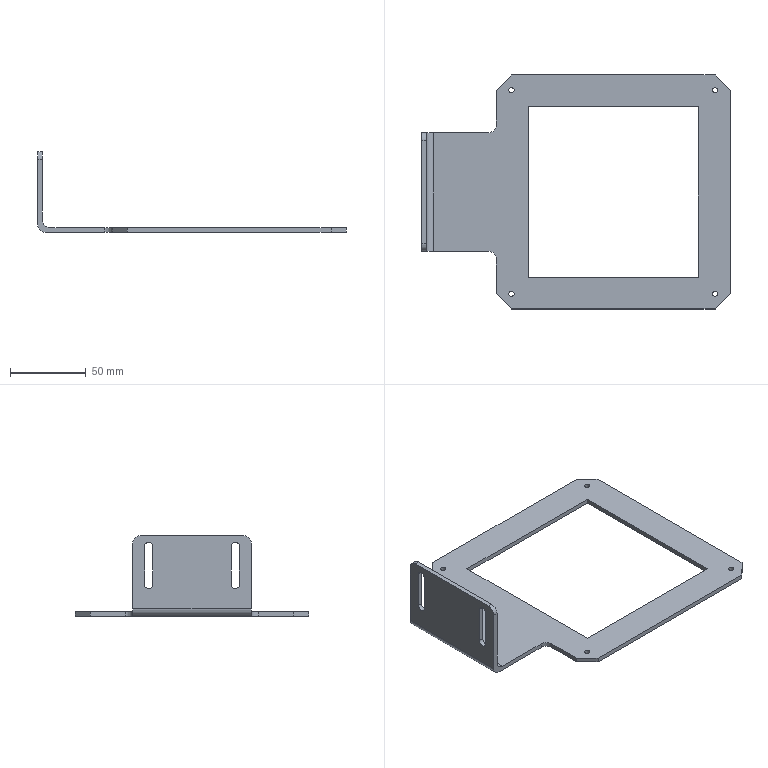Part | STEP file | 11-FG-S02711 | 1 solid | 44 faces | box 203 x 154 x 53 mm | volume 54999 mm3 | plane 24 | cylinder 20 | commonest cylinder face diameters 3.5 x8 5.5 x6 10 x6
STEP:
#1=CARTESIAN_POINT('',(145.75,144.,3.));
#2=VERTEX_POINT('',#1);
#3=CARTESIAN_POINT('',(142.25,144.,3.));
#4=VERTEX_POINT('',#3);
#5=CARTESIAN_POINT('',(144.,144.,3.));
#6=DIRECTION('',(0.,0.,-1.));
#7=DIRECTION('',(-1.,0.,0.));
#8=AXIS2_PLACEMENT_3D('',#5,#6,#7);
#9=CIRCLE('',#8,1.75);
#10=EDGE_CURVE('',#2,#4,#9,.T.);
#11=ORIENTED_EDGE('',*,*,#10,.F.);
#12=CARTESIAN_POINT('',(145.75,144.,0.));
#13=VERTEX_POINT('',#12);
#14=CARTESIAN_POINT('',(145.75,144.,10.));
#15=DIRECTION('',(0.,0.,-1.));
#16=VECTOR('',#15,1000.);
#17=LINE('',#14,#16);
#18=EDGE_CURVE('',#2,#13,#17,.T.);
#19=ORIENTED_EDGE('',*,*,#18,.T.);
#20=CARTESIAN_POINT('',(142.25,144.,0.));
#21=VERTEX_POINT('',#20);
#22=CARTESIAN_POINT('',(144.,144.,0.));
#23=DIRECTION('',(0.,0.,-1.));
#24=DIRECTION('',(-1.,0.,0.));
#25=AXIS2_PLACEMENT_3D('',#22,#23,#24);
#26=CIRCLE('',#25,1.75);
#27=EDGE_CURVE('',#13,#21,#26,.T.);
#28=ORIENTED_EDGE('',*,*,#27,.T.);
#29=CARTESIAN_POINT('',(142.25,144.,10.));
#30=DIRECTION('',(0.,0.,-1.));
#31=VECTOR('',#30,1000.);
#32=LINE('',#29,#31);
#33=EDGE_CURVE('',#4,#21,#32,.T.);
#34=ORIENTED_EDGE('',*,*,#33,.F.);
#35=EDGE_LOOP('',(#11,#19,#28,#34));
#36=FACE_OUTER_BOUND('',#35,.T.);
#37=CARTESIAN_POINT('',(144.,144.,10.));
#38=DIRECTION('',(0.,0.,-1.));
#39=DIRECTION('',(-1.,0.,0.));
#40=AXIS2_PLACEMENT_3D('',#37,#38,#39);
#41=CYLINDRICAL_SURFACE('',#40,1.75);
#42=ADVANCED_FACE('',(#36),#41,.F.);
#43=CARTESIAN_POINT('',(145.75,10.,3.));
#44=VERTEX_POINT('',#43);
#45=CARTESIAN_POINT('',(142.25,10.,3.));
#46=VERTEX_POINT('',#45);
#47=CARTESIAN_POINT('',(144.,10.,3.));
#48=DIRECTION('',(0.,0.,-1.));
#49=DIRECTION('',(-1.,0.,0.));
#50=AXIS2_PLACEMENT_3D('',#47,#48,#49);
#51=CIRCLE('',#50,1.75);
#52=EDGE_CURVE('',#44,#46,#51,.T.);
#53=ORIENTED_EDGE('',*,*,#52,.F.);
#54=CARTESIAN_POINT('',(145.75,10.,0.));
#55=VERTEX_POINT('',#54);
#56=CARTESIAN_POINT('',(145.75,10.,10.));
#57=DIRECTION('',(0.,0.,-1.));
#58=VECTOR('',#57,1000.);
#59=LINE('',#56,#58);
#60=EDGE_CURVE('',#44,#55,#59,.T.);
#61=ORIENTED_EDGE('',*,*,#60,.T.);
#62=CARTESIAN_POINT('',(142.25,10.,0.));
#63=VERTEX_POINT('',#62);
#64=CARTESIAN_POINT('',(144.,10.,0.));
#65=DIRECTION('',(0.,0.,-1.));
#66=DIRECTION('',(-1.,0.,0.));
#67=AXIS2_PLACEMENT_3D('',#64,#65,#66);
#68=CIRCLE('',#67,1.75);
#69=EDGE_CURVE('',#55,#63,#68,.T.);
#70=ORIENTED_EDGE('',*,*,#69,.T.);
#71=CARTESIAN_POINT('',(142.25,10.,10.));
#72=DIRECTION('',(0.,0.,-1.));
#73=VECTOR('',#72,1000.);
#74=LINE('',#71,#73);
#75=EDGE_CURVE('',#46,#63,#74,.T.);
#76=ORIENTED_EDGE('',*,*,#75,.F.);
#77=EDGE_LOOP('',(#53,#61,#70,#76));
#78=FACE_OUTER_BOUND('',#77,.T.);
#79=CARTESIAN_POINT('',(144.,10.,10.));
#80=DIRECTION('',(0.,0.,-1.));
#81=DIRECTION('',(-1.,0.,0.));
#82=AXIS2_PLACEMENT_3D('',#79,#80,#81);
#83=CYLINDRICAL_SURFACE('',#82,1.75);
#84=ADVANCED_FACE('',(#78),#83,.F.);
#85=CARTESIAN_POINT('',(11.75,10.,3.));
#86=VERTEX_POINT('',#85);
#87=CARTESIAN_POINT('',(8.25,10.,3.));
#88=VERTEX_POINT('',#87);
#89=CARTESIAN_POINT('',(10.,10.,3.));
#90=DIRECTION('',(0.,0.,-1.));
#91=DIRECTION('',(-1.,0.,0.));
#92=AXIS2_PLACEMENT_3D('',#89,#90,#91);
#93=CIRCLE('',#92,1.75);
#94=EDGE_CURVE('',#86,#88,#93,.T.);
#95=ORIENTED_EDGE('',*,*,#94,.F.);
#96=CARTESIAN_POINT('',(11.75,10.,0.));
#97=VERTEX_POINT('',#96);
#98=CARTESIAN_POINT('',(11.75,10.,10.));
#99=DIRECTION('',(0.,0.,-1.));
#100=VECTOR('',#99,1000.);
#101=LINE('',#98,#100);
#102=EDGE_CURVE('',#86,#97,#101,.T.);
#103=ORIENTED_EDGE('',*,*,#102,.T.);
#104=CARTESIAN_POINT('',(8.25,10.,0.));
#105=VERTEX_POINT('',#104);
#106=CARTESIAN_POINT('',(10.,10.,0.));
#107=DIRECTION('',(0.,0.,-1.));
#108=DIRECTION('',(-1.,0.,0.));
#109=AXIS2_PLACEMENT_3D('',#106,#107,#108);
#110=CIRCLE('',#109,1.75);
#111=EDGE_CURVE('',#97,#105,#110,.T.);
#112=ORIENTED_EDGE('',*,*,#111,.T.);
#113=CARTESIAN_POINT('',(8.25,10.,10.));
#114=DIRECTION('',(0.,0.,-1.));
#115=VECTOR('',#114,1000.);
#116=LINE('',#113,#115);
#117=EDGE_CURVE('',#88,#105,#116,.T.);
#118=ORIENTED_EDGE('',*,*,#117,.F.);
#119=EDGE_LOOP('',(#95,#103,#112,#118));
#120=FACE_OUTER_BOUND('',#119,.T.);
#121=CARTESIAN_POINT('',(10.,10.,10.));
#122=DIRECTION('',(0.,0.,-1.));
#123=DIRECTION('',(-1.,0.,0.));
#124=AXIS2_PLACEMENT_3D('',#121,#122,#123);
#125=CYLINDRICAL_SURFACE('',#124,1.75);
#126=ADVANCED_FACE('',(#120),#125,.F.);
#127=CARTESIAN_POINT('',(11.75,144.,3.));
#128=VERTEX_POINT('',#127);
#129=CARTESIAN_POINT('',(8.25,144.,3.));
#130=VERTEX_POINT('',#129);
#131=CARTESIAN_POINT('',(10.,144.,3.));
#132=DIRECTION('',(0.,0.,-1.));
#133=DIRECTION('',(-1.,0.,0.));
#134=AXIS2_PLACEMENT_3D('',#131,#132,#133);
#135=CIRCLE('',#134,1.75);
#136=EDGE_CURVE('',#128,#130,#135,.T.);
#137=ORIENTED_EDGE('',*,*,#136,.F.);
#138=CARTESIAN_POINT('',(11.75,144.,0.));
#139=VERTEX_POINT('',#138);
#140=CARTESIAN_POINT('',(11.75,144.,10.));
#141=DIRECTION('',(0.,0.,-1.));
#142=VECTOR('',#141,1000.);
#143=LINE('',#140,#142);
#144=EDGE_CURVE('',#128,#139,#143,.T.);
#145=ORIENTED_EDGE('',*,*,#144,.T.);
#146=CARTESIAN_POINT('',(8.25,144.,0.));
#147=VERTEX_POINT('',#146);
#148=CARTESIAN_POINT('',(10.,144.,0.));
#149=DIRECTION('',(0.,0.,-1.));
#150=DIRECTION('',(-1.,0.,0.));
#151=AXIS2_PLACEMENT_3D('',#148,#149,#150);
#152=CIRCLE('',#151,1.75);
#153=EDGE_CURVE('',#139,#147,#152,.T.);
#154=ORIENTED_EDGE('',*,*,#153,.T.);
#155=CARTESIAN_POINT('',(8.25,144.,10.));
#156=DIRECTION('',(0.,0.,-1.));
#157=VECTOR('',#156,1000.);
#158=LINE('',#155,#157);
#159=EDGE_CURVE('',#130,#147,#158,.T.);
#160=ORIENTED_EDGE('',*,*,#159,.F.);
#161=EDGE_LOOP('',(#137,#145,#154,#160));
#162=FACE_OUTER_BOUND('',#161,.T.);
#163=CARTESIAN_POINT('',(10.,144.,10.));
#164=DIRECTION('',(0.,0.,-1.));
#165=DIRECTION('',(-1.,0.,0.));
#166=AXIS2_PLACEMENT_3D('',#163,#164,#165);
#167=CYLINDRICAL_SURFACE('',#166,1.75);
#168=ADVANCED_FACE('',(#162),#167,.F.);
#169=CARTESIAN_POINT('',(-46.,105.5,48.75));
#170=VERTEX_POINT('',#169);
#171=CARTESIAN_POINT('',(-46.,108.25,46.));
#172=VERTEX_POINT('',#171);
#173=CARTESIAN_POINT('',(-46.,105.5,46.));
#174=DIRECTION('',(-1.,0.,0.));
#175=DIRECTION('',(0.,0.,1.));
#176=AXIS2_PLACEMENT_3D('',#173,#174,#175);
#177=CIRCLE('',#176,2.75);
#178=EDGE_CURVE('',#170,#172,#177,.T.);
#179=ORIENTED_EDGE('',*,*,#178,.F.);
#180=CARTESIAN_POINT('',(-49.,105.5,48.75));
#181=VERTEX_POINT('',#180);
#182=CARTESIAN_POINT('',(1.,105.5,48.75));
#183=DIRECTION('',(-1.,0.,0.));
#184=VECTOR('',#183,1000.);
#185=LINE('',#182,#184);
#186=EDGE_CURVE('',#170,#181,#185,.T.);
#187=ORIENTED_EDGE('',*,*,#186,.T.);
#188=CARTESIAN_POINT('',(-49.,108.25,46.));
#189=VERTEX_POINT('',#188);
#190=CARTESIAN_POINT('',(-49.,105.5,46.));
#191=DIRECTION('',(-1.,0.,0.));
#192=DIRECTION('',(0.,0.,1.));
#193=AXIS2_PLACEMENT_3D('',#190,#191,#192);
#194=CIRCLE('',#193,2.75);
#195=EDGE_CURVE('',#181,#189,#194,.T.);
#196=ORIENTED_EDGE('',*,*,#195,.T.);
#197=CARTESIAN_POINT('',(1.,108.25,46.));
#198=DIRECTION('',(-1.,0.,0.));
#199=VECTOR('',#198,1000.);
#200=LINE('',#197,#199);
#201=EDGE_CURVE('',#172,#189,#200,.T.);
#202=ORIENTED_EDGE('',*,*,#201,.F.);
#203=EDGE_LOOP('',(#179,#187,#196,#202));
#204=FACE_OUTER_BOUND('',#203,.T.);
#205=CARTESIAN_POINT('',(1.,105.5,46.));
#206=DIRECTION('',(-1.,0.,0.));
#207=DIRECTION('',(0.,0.,1.));
#208=AXIS2_PLACEMENT_3D('',#205,#206,#207);
#209=CYLINDRICAL_SURFACE('',#208,2.75);
#210=ADVANCED_FACE('',(#204),#209,.F.);
#211=CARTESIAN_POINT('',(-46.,48.5,48.75));
#212=VERTEX_POINT('',#211);
#213=CARTESIAN_POINT('',(-46.,51.25,46.));
#214=VERTEX_POINT('',#213);
#215=CARTESIAN_POINT('',(-46.,48.5,46.));
#216=DIRECTION('',(-1.,0.,0.));
#217=DIRECTION('',(0.,0.,1.));
#218=AXIS2_PLACEMENT_3D('',#215,#216,#217);
#219=CIRCLE('',#218,2.75);
#220=EDGE_CURVE('',#212,#214,#219,.T.);
#221=ORIENTED_EDGE('',*,*,#220,.F.);
#222=CARTESIAN_POINT('',(-49.,48.5,48.75));
#223=VERTEX_POINT('',#222);
#224=CARTESIAN_POINT('',(1.,48.5,48.75));
#225=DIRECTION('',(-1.,0.,0.));
#226=VECTOR('',#225,1000.);
#227=LINE('',#224,#226);
#228=EDGE_CURVE('',#212,#223,#227,.T.);
#229=ORIENTED_EDGE('',*,*,#228,.T.);
#230=CARTESIAN_POINT('',(-49.,51.25,46.));
#231=VERTEX_POINT('',#230);
#232=CARTESIAN_POINT('',(-49.,48.5,46.));
#233=DIRECTION('',(-1.,0.,0.));
#234=DIRECTION('',(0.,0.,1.));
#235=AXIS2_PLACEMENT_3D('',#232,#233,#234);
#236=CIRCLE('',#235,2.75);
#237=EDGE_CURVE('',#223,#231,#236,.T.);
#238=ORIENTED_EDGE('',*,*,#237,.T.);
#239=CARTESIAN_POINT('',(1.,51.25,46.));
#240=DIRECTION('',(-1.,0.,0.));
#241=VECTOR('',#240,1000.);
#242=LINE('',#239,#241);
#243=EDGE_CURVE('',#214,#231,#242,.T.);
#244=ORIENTED_EDGE('',*,*,#243,.F.);
#245=EDGE_LOOP('',(#221,#229,#238,#244));
#246=FACE_OUTER_BOUND('',#245,.T.);
#247=CARTESIAN_POINT('',(1.,48.5,46.));
#248=DIRECTION('',(-1.,0.,0.));
#249=DIRECTION('',(0.,0.,1.));
#250=AXIS2_PLACEMENT_3D('',#247,#248,#249);
#251=CYLINDRICAL_SURFACE('',#250,2.75);
#252=ADVANCED_FACE('',(#246),#251,.F.);
#253=CARTESIAN_POINT('',(144.,144.,3.));
#254=DIRECTION('',(0.,0.,-1.));
#255=DIRECTION('',(-1.,0.,0.));
#256=AXIS2_PLACEMENT_3D('',#253,#254,#255);
#257=CIRCLE('',#256,1.75);
#258=EDGE_CURVE('',#4,#2,#257,.T.);
#259=ORIENTED_EDGE('',*,*,#258,.T.);
#260=ORIENTED_EDGE('',*,*,#10,.T.);
#261=EDGE_LOOP('',(#259,#260));
#262=FACE_BOUND('',#261,.T.);
#263=CARTESIAN_POINT('',(144.,10.,3.));
#264=DIRECTION('',(0.,0.,-1.));
#265=DIRECTION('',(-1.,0.,0.));
#266=AXIS2_PLACEMENT_3D('',#263,#264,#265);
#267=CIRCLE('',#266,1.75);
#268=EDGE_CURVE('',#46,#44,#267,.T.);
#269=ORIENTED_EDGE('',*,*,#268,.T.);
#270=ORIENTED_EDGE('',*,*,#52,.T.);
#271=EDGE_LOOP('',(#269,#270));
#272=FACE_BOUND('',#271,.T.);
#273=CARTESIAN_POINT('',(10.,10.,3.));
#274=DIRECTION('',(0.,0.,-1.));
#275=DIRECTION('',(-1.,0.,0.));
#276=AXIS2_PLACEMENT_3D('',#273,#274,#275);
#277=CIRCLE('',#276,1.75);
#278=EDGE_CURVE('',#88,#86,#277,.T.);
#279=ORIENTED_EDGE('',*,*,#278,.T.);
#280=ORIENTED_EDGE('',*,*,#94,.T.);
#281=EDGE_LOOP('',(#279,#280));
#282=FACE_BOUND('',#281,.T.);
#283=CARTESIAN_POINT('',(10.,144.,3.));
#284=DIRECTION('',(0.,0.,-1.));
#285=DIRECTION('',(-1.,0.,0.));
#286=AXIS2_PLACEMENT_3D('',#283,#284,#285);
#287=CIRCLE('',#286,1.75);
#288=EDGE_CURVE('',#130,#128,#287,.T.);
#289=ORIENTED_EDGE('',*,*,#288,.T.);
#290=ORIENTED_EDGE('',*,*,#136,.T.);
#291=EDGE_LOOP('',(#289,#290));
#292=FACE_BOUND('',#291,.T.);
#293=CARTESIAN_POINT('',(21.,133.,3.));
#294=VERTEX_POINT('',#293);
#295=CARTESIAN_POINT('',(21.,21.,3.));
#296=VERTEX_POINT('',#295);
#297=CARTESIAN_POINT('',(21.,21.,3.));
#298=DIRECTION('',(0.,-1.,0.));
#299=VECTOR('',#298,1000.);
#300=LINE('',#297,#299);
#301=EDGE_CURVE('',#294,#296,#300,.T.);
#302=ORIENTED_EDGE('',*,*,#301,.F.);
#303=CARTESIAN_POINT('',(133.,133.,3.));
#304=VERTEX_POINT('',#303);
#305=CARTESIAN_POINT('',(21.,133.,3.));
#306=DIRECTION('',(-1.,0.,0.));
#307=VECTOR('',#306,1000.);
#308=LINE('',#305,#307);
#309=EDGE_CURVE('',#304,#294,#308,.T.);
#310=ORIENTED_EDGE('',*,*,#309,.F.);
#311=CARTESIAN_POINT('',(133.,21.,3.));
#312=VERTEX_POINT('',#311);
#313=CARTESIAN_POINT('',(133.,21.,3.));
#314=DIRECTION('',(0.,1.,0.));
#315=VECTOR('',#314,1000.);
#316=LINE('',#313,#315);
#317=EDGE_CURVE('',#312,#304,#316,.T.);
#318=ORIENTED_EDGE('',*,*,#317,.F.);
#319=CARTESIAN_POINT('',(21.,21.,3.));
#320=DIRECTION('',(1.,0.,0.));
#321=VECTOR('',#320,1000.);
#322=LINE('',#319,#321);
#323=EDGE_CURVE('',#296,#312,#322,.T.);
#324=ORIENTED_EDGE('',*,*,#323,.F.);
#325=EDGE_LOOP('',(#302,#310,#318,#324));
#326=FACE_BOUND('',#325,.T.);
#327=CARTESIAN_POINT('',(-41.,116.,3.));
#328=VERTEX_POINT('',#327);
#329=CARTESIAN_POINT('',(-5.,116.,3.));
#330=VERTEX_POINT('',#329);
#331=CARTESIAN_POINT('',(-49.,116.,3.));
#332=DIRECTION('',(1.,0.,0.));
#333=VECTOR('',#332,1000.);
#334=LINE('',#331,#333);
#335=EDGE_CURVE('',#328,#330,#334,.T.);
#336=ORIENTED_EDGE('',*,*,#335,.F.);
#337=CARTESIAN_POINT('',(-41.,38.,3.));
#338=VERTEX_POINT('',#337);
#339=CARTESIAN_POINT('',(-41.,38.,3.));
#340=DIRECTION('',(0.,-1.,0.));
#341=VECTOR('',#340,1000.);
#342=LINE('',#339,#341);
#343=EDGE_CURVE('',#328,#338,#342,.T.);
#344=ORIENTED_EDGE('',*,*,#343,.T.);
#345=CARTESIAN_POINT('',(-5.,38.,3.));
#346=VERTEX_POINT('',#345);
#347=CARTESIAN_POINT('',(-49.,38.,3.));
#348=DIRECTION('',(1.,0.,0.));
#349=VECTOR('',#348,1000.);
#350=LINE('',#347,#349);
#351=EDGE_CURVE('',#338,#346,#350,.T.);
#352=ORIENTED_EDGE('',*,*,#351,.T.);
#353=CARTESIAN_POINT('',(0.,33.,3.));
#354=VERTEX_POINT('',#353);
#355=CARTESIAN_POINT('',(-5.,33.,3.));
#356=DIRECTION('',(0.,0.,-1.));
#357=DIRECTION('',(-1.,0.,0.));
#358=AXIS2_PLACEMENT_3D('',#355,#356,#357);
#359=CIRCLE('',#358,5.);
#360=EDGE_CURVE('',#346,#354,#359,.T.);
#361=ORIENTED_EDGE('',*,*,#360,.T.);
#362=CARTESIAN_POINT('',(0.,10.,3.));
#363=VERTEX_POINT('',#362);
#364=CARTESIAN_POINT('',(0.,0.,3.));
#365=DIRECTION('',(0.,-1.,0.));
#366=VECTOR('',#365,1000.);
#367=LINE('',#364,#366);
#368=EDGE_CURVE('',#354,#363,#367,.T.);
#369=ORIENTED_EDGE('',*,*,#368,.T.);
#370=CARTESIAN_POINT('',(10.,0.,3.));
#371=VERTEX_POINT('',#370);
#372=CARTESIAN_POINT('',(10.,0.,3.));
#373=DIRECTION('',(0.7071,-0.7071,0.));
#374=VECTOR('',#373,1000.);
#375=LINE('',#372,#374);
#376=EDGE_CURVE('',#363,#371,#375,.T.);
#377=ORIENTED_EDGE('',*,*,#376,.T.);
#378=CARTESIAN_POINT('',(144.,0.,3.));
#379=VERTEX_POINT('',#378);
#380=CARTESIAN_POINT('',(0.,0.,3.));
#381=DIRECTION('',(1.,0.,0.));
#382=VECTOR('',#381,1000.);
#383=LINE('',#380,#382);
#384=EDGE_CURVE('',#371,#379,#383,.T.);
#385=ORIENTED_EDGE('',*,*,#384,.T.);
#386=CARTESIAN_POINT('',(154.,10.,3.));
#387=VERTEX_POINT('',#386);
#388=CARTESIAN_POINT('',(154.,10.,3.));
#389=DIRECTION('',(0.7071,0.7071,0.));
#390=VECTOR('',#389,1000.);
#391=LINE('',#388,#390);
#392=EDGE_CURVE('',#379,#387,#391,.T.);
#393=ORIENTED_EDGE('',*,*,#392,.T.);
#394=CARTESIAN_POINT('',(154.,144.,3.));
#395=VERTEX_POINT('',#394);
#396=CARTESIAN_POINT('',(154.,0.,3.));
#397=DIRECTION('',(0.,1.,0.));
#398=VECTOR('',#397,1000.);
#399=LINE('',#396,#398);
#400=EDGE_CURVE('',#387,#395,#399,.T.);
#401=ORIENTED_EDGE('',*,*,#400,.T.);
#402=CARTESIAN_POINT('',(144.,154.,3.));
#403=VERTEX_POINT('',#402);
#404=CARTESIAN_POINT('',(144.,154.,3.));
#405=DIRECTION('',(-0.7071,0.7071,0.));
#406=VECTOR('',#405,1000.);
#407=LINE('',#404,#406);
#408=EDGE_CURVE('',#395,#403,#407,.T.);
#409=ORIENTED_EDGE('',*,*,#408,.T.);
#410=CARTESIAN_POINT('',(10.,154.,3.));
#411=VERTEX_POINT('',#410);
#412=CARTESIAN_POINT('',(0.,154.,3.));
#413=DIRECTION('',(-1.,0.,0.));
#414=VECTOR('',#413,1000.);
#415=LINE('',#412,#414);
#416=EDGE_CURVE('',#403,#411,#415,.T.);
#417=ORIENTED_EDGE('',*,*,#416,.T.);
#418=CARTESIAN_POINT('',(0.,144.,3.));
#419=VERTEX_POINT('',#418);
#420=CARTESIAN_POINT('',(0.,144.,3.));
#421=DIRECTION('',(-0.7071,-0.7071,0.));
#422=VECTOR('',#421,1000.);
#423=LINE('',#420,#422);
#424=EDGE_CURVE('',#411,#419,#423,.T.);
#425=ORIENTED_EDGE('',*,*,#424,.T.);
#426=CARTESIAN_POINT('',(0.,121.,3.));
#427=VERTEX_POINT('',#426);
#428=CARTESIAN_POINT('',(0.,0.,3.));
#429=DIRECTION('',(0.,-1.,0.));
#430=VECTOR('',#429,1000.);
#431=LINE('',#428,#430);
#432=EDGE_CURVE('',#419,#427,#431,.T.);
#433=ORIENTED_EDGE('',*,*,#432,.T.);
#434=CARTESIAN_POINT('',(-5.,121.,3.));
#435=DIRECTION('',(0.,0.,-1.));
#436=DIRECTION('',(-1.,0.,0.));
#437=AXIS2_PLACEMENT_3D('',#434,#435,#436);
#438=CIRCLE('',#437,5.);
#439=EDGE_CURVE('',#427,#330,#438,.T.);
#440=ORIENTED_EDGE('',*,*,#439,.T.);
#441=EDGE_LOOP('',(#336,#344,#352,#361,#369,#377,#385,#393,#401,#409,#417,#425,#433,#440));
#442=FACE_OUTER_BOUND('',#441,.T.);
#443=CARTESIAN_POINT('',(0.,0.,3.));
#444=DIRECTION('',(0.,0.,-1.));
#445=DIRECTION('',(-1.,0.,0.));
#446=AXIS2_PLACEMENT_3D('',#443,#444,#445);
#447=PLANE('',#446);
#448=ADVANCED_FACE('',(#262,#272,#282,#292,#326,#442),#447,.F.);
#449=CARTESIAN_POINT('',(0.,144.,0.));
#450=VERTEX_POINT('',#449);
#451=CARTESIAN_POINT('',(0.,121.,0.));
#452=VERTEX_POINT('',#451);
#453=CARTESIAN_POINT('',(0.,0.,0.));
#454=DIRECTION('',(0.,-1.,0.));
#455=VECTOR('',#454,1000.);
#456=LINE('',#453,#455);
#457=EDGE_CURVE('',#450,#452,#456,.T.);
#458=ORIENTED_EDGE('',*,*,#457,.T.);
#459=CARTESIAN_POINT('',(0.,121.,3.));
#460=DIRECTION('',(0.,0.,1.));
#461=VECTOR('',#460,1000.);
#462=LINE('',#459,#461);
#463=EDGE_CURVE('',#452,#427,#462,.T.);
#464=ORIENTED_EDGE('',*,*,#463,.T.);
#465=ORIENTED_EDGE('',*,*,#432,.F.);
#466=CARTESIAN_POINT('',(0.,144.,3.));
#467=DIRECTION('',(0.,0.,-1.));
#468=VECTOR('',#467,1000.);
#469=LINE('',#466,#468);
#470=EDGE_CURVE('',#419,#450,#469,.T.);
#471=ORIENTED_EDGE('',*,*,#470,.T.);
#472=EDGE_LOOP('',(#458,#464,#465,#471));
#473=FACE_OUTER_BOUND('',#472,.T.);
#474=CARTESIAN_POINT('',(0.,0.,3.));
#475=DIRECTION('',(1.,0.,0.));
#476=DIRECTION('',(0.,0.,-1.));
#477=AXIS2_PLACEMENT_3D('',#474,#475,#476);
#478=PLANE('',#477);
#479=ADVANCED_FACE('',(#473),#478,.F.);
#480=ORIENTED_EDGE('',*,*,#368,.F.);
#481=CARTESIAN_POINT('',(0.,33.,0.));
#482=VERTEX_POINT('',#481);
#483=CARTESIAN_POINT('',(0.,33.,0.));
#484=DIRECTION('',(0.,0.,-1.));
#485=VECTOR('',#484,1000.);
#486=LINE('',#483,#485);
#487=EDGE_CURVE('',#354,#482,#486,.T.);
#488=ORIENTED_EDGE('',*,*,#487,.T.);
#489=CARTESIAN_POINT('',(0.,10.,0.));
#490=VERTEX_POINT('',#489);
#491=CARTESIAN_POINT('',(0.,0.,0.));
#492=DIRECTION('',(0.,-1.,0.));
#493=VECTOR('',#492,1000.);
#494=LINE('',#491,#493);
#495=EDGE_CURVE('',#482,#490,#494,.T.);
#496=ORIENTED_EDGE('',*,*,#495,.T.);
#497=CARTESIAN_POINT('',(0.,10.,3.));
#498=DIRECTION('',(0.,0.,1.));
#499=VECTOR('',#498,1000.);
#500=LINE('',#497,#499);
#501=EDGE_CURVE('',#490,#363,#500,.T.);
#502=ORIENTED_EDGE('',*,*,#501,.T.);
#503=EDGE_LOOP('',(#480,#488,#496,#502));
#504=FACE_OUTER_BOUND('',#503,.T.);
#505=CARTESIAN_POINT('',(0.,0.,3.));
#506=DIRECTION('',(1.,0.,0.));
#507=DIRECTION('',(0.,0.,-1.));
#508=AXIS2_PLACEMENT_3D('',#505,#506,#507);
#509=PLANE('',#508);
#510=ADVANCED_FACE('',(#504),#509,.F.);
#511=CARTESIAN_POINT('',(144.,144.,0.));
#512=DIRECTION('',(0.,0.,-1.));
#513=DIRECTION('',(-1.,0.,0.));
#514=AXIS2_PLACEMENT_3D('',#511,#512,#513);
#515=CIRCLE('',#514,1.75);
#516=EDGE_CURVE('',#21,#13,#515,.T.);
#517=ORIENTED_EDGE('',*,*,#516,.F.);
#518=ORIENTED_EDGE('',*,*,#27,.F.);
#519=EDGE_LOOP('',(#517,#518));
#520=FACE_BOUND('',#519,.T.);
#521=CARTESIAN_POINT('',(144.,10.,0.));
#522=DIRECTION('',(0.,0.,-1.));
#523=DIRECTION('',(-1.,0.,0.));
#524=AXIS2_PLACEMENT_3D('',#521,#522,#523);
#525=CIRCLE('',#524,1.75);
#526=EDGE_CURVE('',#63,#55,#525,.T.);
#527=ORIENTED_EDGE('',*,*,#526,.F.);
#528=ORIENTED_EDGE('',*,*,#69,.F.);
#529=EDGE_LOOP('',(#527,#528));
#530=FACE_BOUND('',#529,.T.);
#531=CARTESIAN_POINT('',(10.,10.,0.));
#532=DIRECTION('',(0.,0.,-1.));
#533=DIRECTION('',(-1.,0.,0.));
#534=AXIS2_PLACEMENT_3D('',#531,#532,#533);
#535=CIRCLE('',#534,1.75);
#536=EDGE_CURVE('',#105,#97,#535,.T.);
#537=ORIENTED_EDGE('',*,*,#536,.F.);
#538=ORIENTED_EDGE('',*,*,#111,.F.);
#539=EDGE_LOOP('',(#537,#538));
#540=FACE_BOUND('',#539,.T.);
#541=CARTESIAN_POINT('',(10.,144.,0.));
#542=DIRECTION('',(0.,0.,-1.));
#543=DIRECTION('',(-1.,0.,0.));
#544=AXIS2_PLACEMENT_3D('',#541,#542,#543);
#545=CIRCLE('',#544,1.75);
#546=EDGE_CURVE('',#147,#139,#545,.T.);
#547=ORIENTED_EDGE('',*,*,#546,.F.);
#548=ORIENTED_EDGE('',*,*,#153,.F.);
#549=EDGE_LOOP('',(#547,#548));
#550=FACE_BOUND('',#549,.T.);
#551=CARTESIAN_POINT('',(-44.,38.,0.));
#552=VERTEX_POINT('',#551);
#553=CARTESIAN_POINT('',(-5.,38.,0.));
#554=VERTEX_POINT('',#553);
#555=CARTESIAN_POINT('',(-49.,38.,0.));
#556=DIRECTION('',(1.,0.,0.));
#557=VECTOR('',#556,1000.);
#558=LINE('',#555,#557);
#559=EDGE_CURVE('',#552,#554,#558,.T.);
#560=ORIENTED_EDGE('',*,*,#559,.F.);
#561=CARTESIAN_POINT('',(-44.,116.,0.));
#562=VERTEX_POINT('',#561);
#563=CARTESIAN_POINT('',(-44.,0.,0.));
#564=DIRECTION('',(0.,1.,0.));
#565=VECTOR('',#564,1000.);
#566=LINE('',#563,#565);
#567=EDGE_CURVE('',#552,#562,#566,.T.);
#568=ORIENTED_EDGE('',*,*,#567,.T.);
#569=CARTESIAN_POINT('',(-5.,116.,0.));
#570=VERTEX_POINT('',#569);
#571=CARTESIAN_POINT('',(-49.,116.,0.));
#572=DIRECTION('',(1.,0.,0.));
#573=VECTOR('',#572,1000.);
#574=LINE('',#571,#573);
#575=EDGE_CURVE('',#562,#570,#574,.T.);
#576=ORIENTED_EDGE('',*,*,#575,.T.);
#577=CARTESIAN_POINT('',(-5.,121.,0.));
#578=DIRECTION('',(0.,0.,1.));
#579=DIRECTION('',(-1.,0.,0.));
#580=AXIS2_PLACEMENT_3D('',#577,#578,#579);
#581=CIRCLE('',#580,5.);
#582=EDGE_CURVE('',#570,#452,#581,.T.);
#583=ORIENTED_EDGE('',*,*,#582,.T.);
#584=ORIENTED_EDGE('',*,*,#457,.F.);
#585=CARTESIAN_POINT('',(10.,154.,0.));
#586=VERTEX_POINT('',#585);
#587=CARTESIAN_POINT('',(-72.,72.,0.));
#588=DIRECTION('',(0.7071,0.7071,0.));
#589=VECTOR('',#588,1000.);
#590=LINE('',#587,#589);
#591=EDGE_CURVE('',#450,#586,#590,.T.);
#592=ORIENTED_EDGE('',*,*,#591,.T.);
#593=CARTESIAN_POINT('',(144.,154.,0.));
#594=VERTEX_POINT('',#593);
#595=CARTESIAN_POINT('',(0.,154.,0.));
#596=DIRECTION('',(-1.,0.,0.));
#597=VECTOR('',#596,1000.);
#598=LINE('',#595,#597);
#599=EDGE_CURVE('',#594,#586,#598,.T.);
#600=ORIENTED_EDGE('',*,*,#599,.F.);
#601=CARTESIAN_POINT('',(154.,144.,0.));
#602=VERTEX_POINT('',#601);
#603=CARTESIAN_POINT('',(149.,149.,0.));
#604=DIRECTION('',(0.7071,-0.7071,0.));
#605=VECTOR('',#604,1000.);
#606=LINE('',#603,#605);
#607=EDGE_CURVE('',#594,#602,#606,.T.);
#608=ORIENTED_EDGE('',*,*,#607,.T.);
#609=CARTESIAN_POINT('',(154.,10.,0.));
#610=VERTEX_POINT('',#609);
#611=CARTESIAN_POINT('',(154.,0.,0.));
#612=DIRECTION('',(0.,1.,0.));
#613=VECTOR('',#612,1000.);
#614=LINE('',#611,#613);
#615=EDGE_CURVE('',#610,#602,#614,.T.);
#616=ORIENTED_EDGE('',*,*,#615,.F.);
#617=CARTESIAN_POINT('',(144.,0.,0.));
#618=VERTEX_POINT('',#617);
#619=CARTESIAN_POINT('',(72.,-72.,0.));
#620=DIRECTION('',(-0.7071,-0.7071,0.));
#621=VECTOR('',#620,1000.);
#622=LINE('',#619,#621);
#623=EDGE_CURVE('',#610,#618,#622,.T.);
#624=ORIENTED_EDGE('',*,*,#623,.T.);
#625=CARTESIAN_POINT('',(10.,0.,0.));
#626=VERTEX_POINT('',#625);
#627=CARTESIAN_POINT('',(0.,0.,0.));
#628=DIRECTION('',(1.,0.,0.));
#629=VECTOR('',#628,1000.);
#630=LINE('',#627,#629);
#631=EDGE_CURVE('',#626,#618,#630,.T.);
#632=ORIENTED_EDGE('',*,*,#631,.F.);
#633=CARTESIAN_POINT('',(5.,5.,0.));
#634=DIRECTION('',(-0.7071,0.7071,0.));
#635=VECTOR('',#634,1000.);
#636=LINE('',#633,#635);
#637=EDGE_CURVE('',#626,#490,#636,.T.);
#638=ORIENTED_EDGE('',*,*,#637,.T.);
#639=ORIENTED_EDGE('',*,*,#495,.F.);
#640=CARTESIAN_POINT('',(-5.,33.,0.));
#641=DIRECTION('',(0.,0.,1.));
#642=DIRECTION('',(-1.,0.,0.));
#643=AXIS2_PLACEMENT_3D('',#640,#641,#642);
#644=CIRCLE('',#643,5.);
#645=EDGE_CURVE('',#482,#554,#644,.T.);
#646=ORIENTED_EDGE('',*,*,#645,.T.);
#647=EDGE_LOOP('',(#560,#568,#576,#583,#584,#592,#600,#608,#616,#624,#632,#638,#639,#646));
#648=FACE_OUTER_BOUND('',#647,.T.);
#649=CARTESIAN_POINT('',(133.,133.,0.));
#650=VERTEX_POINT('',#649);
#651=CARTESIAN_POINT('',(21.,133.,0.));
#652=VERTEX_POINT('',#651);
#653=CARTESIAN_POINT('',(21.,133.,0.));
#654=DIRECTION('',(-1.,0.,0.));
#655=VECTOR('',#654,1000.);
#656=LINE('',#653,#655);
#657=EDGE_CURVE('',#650,#652,#656,.T.);
#658=ORIENTED_EDGE('',*,*,#657,.T.);
#659=CARTESIAN_POINT('',(21.,21.,0.));
#660=VERTEX_POINT('',#659);
#661=CARTESIAN_POINT('',(21.,21.,0.));
#662=DIRECTION('',(0.,-1.,0.));
#663=VECTOR('',#662,1000.);
#664=LINE('',#661,#663);
#665=EDGE_CURVE('',#652,#660,#664,.T.);
#666=ORIENTED_EDGE('',*,*,#665,.T.);
#667=CARTESIAN_POINT('',(133.,21.,0.));
#668=VERTEX_POINT('',#667);
#669=CARTESIAN_POINT('',(21.,21.,0.));
#670=DIRECTION('',(1.,0.,0.));
#671=VECTOR('',#670,1000.);
#672=LINE('',#669,#671);
#673=EDGE_CURVE('',#660,#668,#672,.T.);
#674=ORIENTED_EDGE('',*,*,#673,.T.);
#675=CARTESIAN_POINT('',(133.,21.,0.));
#676=DIRECTION('',(0.,1.,0.));
#677=VECTOR('',#676,1000.);
#678=LINE('',#675,#677);
#679=EDGE_CURVE('',#668,#650,#678,.T.);
#680=ORIENTED_EDGE('',*,*,#679,.T.);
#681=EDGE_LOOP('',(#658,#666,#674,#680));
#682=FACE_BOUND('',#681,.T.);
#683=CARTESIAN_POINT('',(0.,0.,0.));
#684=DIRECTION('',(0.,0.,-1.));
#685=DIRECTION('',(-1.,0.,0.));
#686=AXIS2_PLACEMENT_3D('',#683,#684,#685);
#687=PLANE('',#686);
#688=ADVANCED_FACE('',(#520,#530,#540,#550,#648,#682),#687,.T.);
#689=ORIENTED_EDGE('',*,*,#384,.F.);
#690=CARTESIAN_POINT('',(10.,0.,3.));
#691=DIRECTION('',(0.,0.,-1.));
#692=VECTOR('',#691,1000.);
#693=LINE('',#690,#692);
#694=EDGE_CURVE('',#371,#626,#693,.T.);
#695=ORIENTED_EDGE('',*,*,#694,.T.);
#696=ORIENTED_EDGE('',*,*,#631,.T.);
#697=CARTESIAN_POINT('',(144.,0.,3.));
#698=DIRECTION('',(0.,0.,1.));
#699=VECTOR('',#698,1000.);
#700=LINE('',#697,#699);
#701=EDGE_CURVE('',#618,#379,#700,.T.);
#702=ORIENTED_EDGE('',*,*,#701,.T.);
#703=EDGE_LOOP('',(#689,#695,#696,#702));
#704=FACE_OUTER_BOUND('',#703,.T.);
#705=CARTESIAN_POINT('',(0.,0.,3.));
#706=DIRECTION('',(0.,1.,0.));
#707=DIRECTION('',(0.,0.,1.));
#708=AXIS2_PLACEMENT_3D('',#705,#706,#707);
#709=PLANE('',#708);
#710=ADVANCED_FACE('',(#704),#709,.F.);
#711=ORIENTED_EDGE('',*,*,#615,.T.);
#712=CARTESIAN_POINT('',(154.,144.,3.));
#713=DIRECTION('',(0.,0.,1.));
#714=VECTOR('',#713,1000.);
#715=LINE('',#712,#714);
#716=EDGE_CURVE('',#602,#395,#715,.T.);
#717=ORIENTED_EDGE('',*,*,#716,.T.);
#718=ORIENTED_EDGE('',*,*,#400,.F.);
#719=CARTESIAN_POINT('',(154.,10.,3.));
#720=DIRECTION('',(0.,0.,-1.));
#721=VECTOR('',#720,1000.);
#722=LINE('',#719,#721);
#723=EDGE_CURVE('',#387,#610,#722,.T.);
#724=ORIENTED_EDGE('',*,*,#723,.T.);
#725=EDGE_LOOP('',(#711,#717,#718,#724));
#726=FACE_OUTER_BOUND('',#725,.T.);
#727=CARTESIAN_POINT('',(154.,0.,3.));
#728=DIRECTION('',(-1.,0.,0.));
#729=DIRECTION('',(0.,0.,1.));
#730=AXIS2_PLACEMENT_3D('',#727,#728,#729);
#731=PLANE('',#730);
#732=ADVANCED_FACE('',(#726),#731,.F.);
#733=ORIENTED_EDGE('',*,*,#599,.T.);
#734=CARTESIAN_POINT('',(10.,154.,3.));
#735=DIRECTION('',(0.,0.,1.));
#736=VECTOR('',#735,1000.);
#737=LINE('',#734,#736);
#738=EDGE_CURVE('',#586,#411,#737,.T.);
#739=ORIENTED_EDGE('',*,*,#738,.T.);
#740=ORIENTED_EDGE('',*,*,#416,.F.);
#741=CARTESIAN_POINT('',(144.,154.,3.));
#742=DIRECTION('',(0.,0.,-1.));
#743=VECTOR('',#742,1000.);
#744=LINE('',#741,#743);
#745=EDGE_CURVE('',#403,#594,#744,.T.);
#746=ORIENTED_EDGE('',*,*,#745,.T.);
#747=EDGE_LOOP('',(#733,#739,#740,#746));
#748=FACE_OUTER_BOUND('',#747,.T.);
#749=CARTESIAN_POINT('',(0.,154.,3.));
#750=DIRECTION('',(0.,-1.,0.));
#751=DIRECTION('',(0.,0.,-1.));
#752=AXIS2_PLACEMENT_3D('',#749,#750,#751);
#753=PLANE('',#752);
#754=ADVANCED_FACE('',(#748),#753,.F.);
#755=ORIENTED_EDGE('',*,*,#665,.F.);
#756=CARTESIAN_POINT('',(21.,133.,3.));
#757=DIRECTION('',(0.,0.,-1.));
#758=VECTOR('',#757,1000.);
#759=LINE('',#756,#758);
#760=EDGE_CURVE('',#294,#652,#759,.T.);
#761=ORIENTED_EDGE('',*,*,#760,.F.);
#762=ORIENTED_EDGE('',*,*,#301,.T.);
#763=CARTESIAN_POINT('',(21.,21.,3.));
#764=DIRECTION('',(0.,0.,-1.));
#765=VECTOR('',#764,1000.);
#766=LINE('',#763,#765);
#767=EDGE_CURVE('',#296,#660,#766,.T.);
#768=ORIENTED_EDGE('',*,*,#767,.T.);
#769=EDGE_LOOP('',(#755,#761,#762,#768));
#770=FACE_OUTER_BOUND('',#769,.T.);
#771=CARTESIAN_POINT('',(21.,21.,3.));
#772=DIRECTION('',(1.,0.,0.));
#773=DIRECTION('',(0.,0.,-1.));
#774=AXIS2_PLACEMENT_3D('',#771,#772,#773);
#775=PLANE('',#774);
#776=ADVANCED_FACE('',(#770),#775,.T.);
#777=ORIENTED_EDGE('',*,*,#673,.F.);
#778=ORIENTED_EDGE('',*,*,#767,.F.);
#779=ORIENTED_EDGE('',*,*,#323,.T.);
#780=CARTESIAN_POINT('',(133.,21.,3.));
#781=DIRECTION('',(0.,0.,-1.));
#782=VECTOR('',#781,1000.);
#783=LINE('',#780,#782);
#784=EDGE_CURVE('',#312,#668,#783,.T.);
#785=ORIENTED_EDGE('',*,*,#784,.T.);
#786=EDGE_LOOP('',(#777,#778,#779,#785));
#787=FACE_OUTER_BOUND('',#786,.T.);
#788=CARTESIAN_POINT('',(21.,21.,3.));
#789=DIRECTION('',(0.,1.,0.));
#790=DIRECTION('',(0.,0.,1.));
#791=AXIS2_PLACEMENT_3D('',#788,#789,#790);
#792=PLANE('',#791);
#793=ADVANCED_FACE('',(#787),#792,.T.);
#794=ORIENTED_EDGE('',*,*,#679,.F.);
#795=ORIENTED_EDGE('',*,*,#784,.F.);
#796=ORIENTED_EDGE('',*,*,#317,.T.);
#797=CARTESIAN_POINT('',(133.,133.,3.));
#798=DIRECTION('',(0.,0.,-1.));
#799=VECTOR('',#798,1000.);
#800=LINE('',#797,#799);
#801=EDGE_CURVE('',#304,#650,#800,.T.);
#802=ORIENTED_EDGE('',*,*,#801,.T.);
#803=EDGE_LOOP('',(#794,#795,#796,#802));
#804=FACE_OUTER_BOUND('',#803,.T.);
#805=CARTESIAN_POINT('',(133.,21.,3.));
#806=DIRECTION('',(-1.,0.,0.));
#807=DIRECTION('',(0.,0.,1.));
#808=AXIS2_PLACEMENT_3D('',#805,#806,#807);
#809=PLANE('',#808);
#810=ADVANCED_FACE('',(#804),#809,.T.);
#811=ORIENTED_EDGE('',*,*,#657,.F.);
#812=ORIENTED_EDGE('',*,*,#801,.F.);
#813=ORIENTED_EDGE('',*,*,#309,.T.);
#814=ORIENTED_EDGE('',*,*,#760,.T.);
#815=EDGE_LOOP('',(#811,#812,#813,#814));
#816=FACE_OUTER_BOUND('',#815,.T.);
#817=CARTESIAN_POINT('',(21.,133.,3.));
#818=DIRECTION('',(0.,-1.,0.));
#819=DIRECTION('',(0.,0.,-1.));
#820=AXIS2_PLACEMENT_3D('',#817,#818,#819);
#821=PLANE('',#820);
#822=ADVANCED_FACE('',(#816),#821,.T.);
#823=CARTESIAN_POINT('',(-46.,38.,48.));
#824=VERTEX_POINT('',#823);
#825=CARTESIAN_POINT('',(-46.,38.,8.));
#826=VERTEX_POINT('',#825);
#827=CARTESIAN_POINT('',(-46.,38.,53.));
#828=DIRECTION('',(0.,0.,-1.));
#829=VECTOR('',#828,1000.);
#830=LINE('',#827,#829);
#831=EDGE_CURVE('',#824,#826,#830,.T.);
#832=ORIENTED_EDGE('',*,*,#831,.F.);
#833=CARTESIAN_POINT('',(-49.,38.,48.));
#834=VERTEX_POINT('',#833);
#835=CARTESIAN_POINT('',(-49.,38.,48.));
#836=DIRECTION('',(-1.,0.,0.));
#837=VECTOR('',#836,1000.);
#838=LINE('',#835,#837);
#839=EDGE_CURVE('',#824,#834,#838,.T.);
#840=ORIENTED_EDGE('',*,*,#839,.T.);
#841=CARTESIAN_POINT('',(-49.,38.,5.));
#842=VERTEX_POINT('',#841);
#843=CARTESIAN_POINT('',(-49.,38.,0.));
#844=DIRECTION('',(0.,0.,1.));
#845=VECTOR('',#844,1000.);
#846=LINE('',#843,#845);
#847=EDGE_CURVE('',#842,#834,#846,.T.);
#848=ORIENTED_EDGE('',*,*,#847,.F.);
#849=CARTESIAN_POINT('',(-44.,38.,5.));
#850=DIRECTION('',(0.,-1.,0.));
#851=DIRECTION('',(0.,0.,1.));
#852=AXIS2_PLACEMENT_3D('',#849,#850,#851);
#853=CIRCLE('',#852,5.);
#854=EDGE_CURVE('',#842,#552,#853,.T.);
#855=ORIENTED_EDGE('',*,*,#854,.T.);
#856=ORIENTED_EDGE('',*,*,#559,.T.);
#857=CARTESIAN_POINT('',(-5.,38.,3.));
#858=DIRECTION('',(0.,0.,1.));
#859=VECTOR('',#858,1000.);
#860=LINE('',#857,#859);
#861=EDGE_CURVE('',#554,#346,#860,.T.);
#862=ORIENTED_EDGE('',*,*,#861,.T.);
#863=ORIENTED_EDGE('',*,*,#351,.F.);
#864=CARTESIAN_POINT('',(-41.,38.,8.));
#865=DIRECTION('',(0.,1.,0.));
#866=DIRECTION('',(0.,0.,1.));
#867=AXIS2_PLACEMENT_3D('',#864,#865,#866);
#868=CIRCLE('',#867,5.);
#869=EDGE_CURVE('',#338,#826,#868,.T.);
#870=ORIENTED_EDGE('',*,*,#869,.T.);
#871=EDGE_LOOP('',(#832,#840,#848,#855,#856,#862,#863,#870));
#872=FACE_OUTER_BOUND('',#871,.T.);
#873=CARTESIAN_POINT('',(-49.,38.,0.));
#874=DIRECTION('',(0.,1.,0.));
#875=DIRECTION('',(0.,0.,1.));
#876=AXIS2_PLACEMENT_3D('',#873,#874,#875);
#877=PLANE('',#876);
#878=ADVANCED_FACE('',(#872),#877,.F.);
#879=CARTESIAN_POINT('',(-49.,116.,48.));
#880=VERTEX_POINT('',#879);
#881=CARTESIAN_POINT('',(-49.,116.,5.));
#882=VERTEX_POINT('',#881);
#883=CARTESIAN_POINT('',(-49.,116.,0.));
#884=DIRECTION('',(0.,0.,-1.));
#885=VECTOR('',#884,1000.);
#886=LINE('',#883,#885);
#887=EDGE_CURVE('',#880,#882,#886,.T.);
#888=ORIENTED_EDGE('',*,*,#887,.F.);
#889=CARTESIAN_POINT('',(-46.,116.,48.));
#890=VERTEX_POINT('',#889);
#891=CARTESIAN_POINT('',(-49.,116.,48.));
#892=DIRECTION('',(1.,0.,0.));
#893=VECTOR('',#892,1000.);
#894=LINE('',#891,#893);
#895=EDGE_CURVE('',#880,#890,#894,.T.);
#896=ORIENTED_EDGE('',*,*,#895,.T.);
#897=CARTESIAN_POINT('',(-46.,116.,8.));
#898=VERTEX_POINT('',#897);
#899=CARTESIAN_POINT('',(-46.,116.,53.));
#900=DIRECTION('',(0.,0.,-1.));
#901=VECTOR('',#900,1000.);
#902=LINE('',#899,#901);
#903=EDGE_CURVE('',#890,#898,#902,.T.);
#904=ORIENTED_EDGE('',*,*,#903,.T.);
#905=CARTESIAN_POINT('',(-41.,116.,8.));
#906=DIRECTION('',(0.,-1.,0.));
#907=DIRECTION('',(0.,0.,-1.));
#908=AXIS2_PLACEMENT_3D('',#905,#906,#907);
#909=CIRCLE('',#908,5.);
#910=EDGE_CURVE('',#898,#328,#909,.T.);
#911=ORIENTED_EDGE('',*,*,#910,.T.);
#912=ORIENTED_EDGE('',*,*,#335,.T.);
#913=CARTESIAN_POINT('',(-5.,116.,0.));
#914=DIRECTION('',(0.,0.,-1.));
#915=VECTOR('',#914,1000.);
#916=LINE('',#913,#915);
#917=EDGE_CURVE('',#330,#570,#916,.T.);
#918=ORIENTED_EDGE('',*,*,#917,.T.);
#919=ORIENTED_EDGE('',*,*,#575,.F.);
#920=CARTESIAN_POINT('',(-44.,116.,5.));
#921=DIRECTION('',(0.,1.,0.));
#922=DIRECTION('',(0.,0.,-1.));
#923=AXIS2_PLACEMENT_3D('',#920,#921,#922);
#924=CIRCLE('',#923,5.);
#925=EDGE_CURVE('',#562,#882,#924,.T.);
#926=ORIENTED_EDGE('',*,*,#925,.T.);
#927=EDGE_LOOP('',(#888,#896,#904,#911,#912,#918,#919,#926));
#928=FACE_OUTER_BOUND('',#927,.T.);
#929=CARTESIAN_POINT('',(-49.,116.,0.));
#930=DIRECTION('',(0.,-1.,0.));
#931=DIRECTION('',(0.,0.,-1.));
#932=AXIS2_PLACEMENT_3D('',#929,#930,#931);
#933=PLANE('',#932);
#934=ADVANCED_FACE('',(#928),#933,.F.);
#935=CARTESIAN_POINT('',(-49.,102.75,46.));
#936=VERTEX_POINT('',#935);
#937=CARTESIAN_POINT('',(-49.,105.5,46.));
#938=DIRECTION('',(-1.,0.,0.));
#939=DIRECTION('',(0.,0.,1.));
#940=AXIS2_PLACEMENT_3D('',#937,#938,#939);
#941=CIRCLE('',#940,2.75);
#942=EDGE_CURVE('',#936,#181,#941,.T.);
#943=ORIENTED_EDGE('',*,*,#942,.F.);
#944=CARTESIAN_POINT('',(-49.,102.75,21.));
#945=VERTEX_POINT('',#944);
#946=CARTESIAN_POINT('',(-49.,102.75,46.));
#947=DIRECTION('',(0.,0.,1.));
#948=VECTOR('',#947,1000.);
#949=LINE('',#946,#948);
#950=EDGE_CURVE('',#945,#936,#949,.T.);
#951=ORIENTED_EDGE('',*,*,#950,.F.);
#952=CARTESIAN_POINT('',(-49.,108.25,21.));
#953=VERTEX_POINT('',#952);
#954=CARTESIAN_POINT('',(-49.,105.5,21.));
#955=DIRECTION('',(-1.,0.,0.));
#956=DIRECTION('',(0.,0.,1.));
#957=AXIS2_PLACEMENT_3D('',#954,#955,#956);
#958=CIRCLE('',#957,2.75);
#959=EDGE_CURVE('',#953,#945,#958,.T.);
#960=ORIENTED_EDGE('',*,*,#959,.F.);
#961=CARTESIAN_POINT('',(-49.,108.25,46.));
#962=DIRECTION('',(0.,0.,-1.));
#963=VECTOR('',#962,1000.);
#964=LINE('',#961,#963);
#965=EDGE_CURVE('',#189,#953,#964,.T.);
#966=ORIENTED_EDGE('',*,*,#965,.F.);
#967=ORIENTED_EDGE('',*,*,#195,.F.);
#968=EDGE_LOOP('',(#943,#951,#960,#966,#967));
#969=FACE_BOUND('',#968,.T.);
#970=CARTESIAN_POINT('',(-49.,45.75,46.));
#971=VERTEX_POINT('',#970);
#972=CARTESIAN_POINT('',(-49.,48.5,46.));
#973=DIRECTION('',(-1.,0.,0.));
#974=DIRECTION('',(0.,0.,1.));
#975=AXIS2_PLACEMENT_3D('',#972,#973,#974);
#976=CIRCLE('',#975,2.75);
#977=EDGE_CURVE('',#971,#223,#976,.T.);
#978=ORIENTED_EDGE('',*,*,#977,.F.);
#979=CARTESIAN_POINT('',(-49.,45.75,21.));
#980=VERTEX_POINT('',#979);
#981=CARTESIAN_POINT('',(-49.,45.75,46.));
#982=DIRECTION('',(0.,0.,1.));
#983=VECTOR('',#982,1000.);
#984=LINE('',#981,#983);
#985=EDGE_CURVE('',#980,#971,#984,.T.);
#986=ORIENTED_EDGE('',*,*,#985,.F.);
#987=CARTESIAN_POINT('',(-49.,51.25,21.));
#988=VERTEX_POINT('',#987);
#989=CARTESIAN_POINT('',(-49.,48.5,21.));
#990=DIRECTION('',(-1.,0.,0.));
#991=DIRECTION('',(0.,0.,1.));
#992=AXIS2_PLACEMENT_3D('',#989,#990,#991);
#993=CIRCLE('',#992,2.75);
#994=EDGE_CURVE('',#988,#980,#993,.T.);
#995=ORIENTED_EDGE('',*,*,#994,.F.);
#996=CARTESIAN_POINT('',(-49.,51.25,46.));
#997=DIRECTION('',(0.,0.,-1.));
#998=VECTOR('',#997,1000.);
#999=LINE('',#996,#998);
#1000=EDGE_CURVE('',#231,#988,#999,.T.);
#1001=ORIENTED_EDGE('',*,*,#1000,.F.);
#1002=ORIENTED_EDGE('',*,*,#237,.F.);
#1003=EDGE_LOOP('',(#978,#986,#995,#1001,#1002));
#1004=FACE_BOUND('',#1003,.T.);
#1005=CARTESIAN_POINT('',(-49.,111.,53.));
#1006=VERTEX_POINT('',#1005);
#1007=CARTESIAN_POINT('',(-49.,43.,53.));
#1008=VERTEX_POINT('',#1007);
#1009=CARTESIAN_POINT('',(-49.,38.,53.));
#1010=DIRECTION('',(0.,-1.,0.));
#1011=VECTOR('',#1010,1000.);
#1012=LINE('',#1009,#1011);
#1013=EDGE_CURVE('',#1006,#1008,#1012,.T.);
#1014=ORIENTED_EDGE('',*,*,#1013,.F.);
#1015=CARTESIAN_POINT('',(-49.,111.,48.));
#1016=DIRECTION('',(-1.,0.,0.));
#1017=DIRECTION('',(0.,0.,1.));
#1018=AXIS2_PLACEMENT_3D('',#1015,#1016,#1017);
#1019=CIRCLE('',#1018,5.);
#1020=EDGE_CURVE('',#1006,#880,#1019,.T.);
#1021=ORIENTED_EDGE('',*,*,#1020,.T.);
#1022=ORIENTED_EDGE('',*,*,#887,.T.);
#1023=CARTESIAN_POINT('',(-49.,0.,5.));
#1024=DIRECTION('',(0.,-1.,0.));
#1025=VECTOR('',#1024,1000.);
#1026=LINE('',#1023,#1025);
#1027=EDGE_CURVE('',#882,#842,#1026,.T.);
#1028=ORIENTED_EDGE('',*,*,#1027,.T.);
#1029=ORIENTED_EDGE('',*,*,#847,.T.);
#1030=CARTESIAN_POINT('',(-49.,43.,48.));
#1031=DIRECTION('',(-1.,0.,0.));
#1032=DIRECTION('',(0.,0.,1.));
#1033=AXIS2_PLACEMENT_3D('',#1030,#1031,#1032);
#1034=CIRCLE('',#1033,5.);
#1035=EDGE_CURVE('',#834,#1008,#1034,.T.);
#1036=ORIENTED_EDGE('',*,*,#1035,.T.);
#1037=EDGE_LOOP('',(#1014,#1021,#1022,#1028,#1029,#1036));
#1038=FACE_OUTER_BOUND('',#1037,.T.);
#1039=CARTESIAN_POINT('',(-49.,0.,0.));
#1040=DIRECTION('',(-1.,0.,0.));
#1041=DIRECTION('',(0.,0.,1.));
#1042=AXIS2_PLACEMENT_3D('',#1039,#1040,#1041);
#1043=PLANE('',#1042);
#1044=ADVANCED_FACE('',(#969,#1004,#1038),#1043,.T.);
#1045=CARTESIAN_POINT('',(-46.,102.75,21.));
#1046=VERTEX_POINT('',#1045);
#1047=CARTESIAN_POINT('',(-46.,102.75,46.));
#1048=VERTEX_POINT('',#1047);
#1049=CARTESIAN_POINT('',(-46.,102.75,53.));
#1050=DIRECTION('',(0.,0.,1.));
#1051=VECTOR('',#1050,1000.);
#1052=LINE('',#1049,#1051);
#1053=EDGE_CURVE('',#1046,#1048,#1052,.T.);
#1054=ORIENTED_EDGE('',*,*,#1053,.T.);
#1055=CARTESIAN_POINT('',(-46.,105.5,46.));
#1056=DIRECTION('',(-1.,0.,0.));
#1057=DIRECTION('',(0.,0.,1.));
#1058=AXIS2_PLACEMENT_3D('',#1055,#1056,#1057);
#1059=CIRCLE('',#1058,2.75);
#1060=EDGE_CURVE('',#1048,#170,#1059,.T.);
#1061=ORIENTED_EDGE('',*,*,#1060,.T.);
#1062=ORIENTED_EDGE('',*,*,#178,.T.);
#1063=CARTESIAN_POINT('',(-46.,108.25,21.));
#1064=VERTEX_POINT('',#1063);
#1065=CARTESIAN_POINT('',(-46.,108.25,53.));
#1066=DIRECTION('',(0.,0.,-1.));
#1067=VECTOR('',#1066,1000.);
#1068=LINE('',#1065,#1067);
#1069=EDGE_CURVE('',#172,#1064,#1068,.T.);
#1070=ORIENTED_EDGE('',*,*,#1069,.T.);
#1071=CARTESIAN_POINT('',(-46.,105.5,21.));
#1072=DIRECTION('',(-1.,0.,0.));
#1073=DIRECTION('',(0.,0.,1.));
#1074=AXIS2_PLACEMENT_3D('',#1071,#1072,#1073);
#1075=CIRCLE('',#1074,2.75);
#1076=EDGE_CURVE('',#1064,#1046,#1075,.T.);
#1077=ORIENTED_EDGE('',*,*,#1076,.T.);
#1078=EDGE_LOOP('',(#1054,#1061,#1062,#1070,#1077));
#1079=FACE_BOUND('',#1078,.T.);
#1080=CARTESIAN_POINT('',(-46.,45.75,21.));
#1081=VERTEX_POINT('',#1080);
#1082=CARTESIAN_POINT('',(-46.,45.75,46.));
#1083=VERTEX_POINT('',#1082);
#1084=CARTESIAN_POINT('',(-46.,45.75,53.));
#1085=DIRECTION('',(0.,0.,1.));
#1086=VECTOR('',#1085,1000.);
#1087=LINE('',#1084,#1086);
#1088=EDGE_CURVE('',#1081,#1083,#1087,.T.);
#1089=ORIENTED_EDGE('',*,*,#1088,.T.);
#1090=CARTESIAN_POINT('',(-46.,48.5,46.));
#1091=DIRECTION('',(-1.,0.,0.));
#1092=DIRECTION('',(0.,0.,1.));
#1093=AXIS2_PLACEMENT_3D('',#1090,#1091,#1092);
#1094=CIRCLE('',#1093,2.75);
#1095=EDGE_CURVE('',#1083,#212,#1094,.T.);
#1096=ORIENTED_EDGE('',*,*,#1095,.T.);
#1097=ORIENTED_EDGE('',*,*,#220,.T.);
#1098=CARTESIAN_POINT('',(-46.,51.25,21.));
#1099=VERTEX_POINT('',#1098);
#1100=CARTESIAN_POINT('',(-46.,51.25,53.));
#1101=DIRECTION('',(0.,0.,-1.));
#1102=VECTOR('',#1101,1000.);
#1103=LINE('',#1100,#1102);
#1104=EDGE_CURVE('',#214,#1099,#1103,.T.);
#1105=ORIENTED_EDGE('',*,*,#1104,.T.);
#1106=CARTESIAN_POINT('',(-46.,48.5,21.));
#1107=DIRECTION('',(-1.,0.,0.));
#1108=DIRECTION('',(0.,0.,1.));
#1109=AXIS2_PLACEMENT_3D('',#1106,#1107,#1108);
#1110=CIRCLE('',#1109,2.75);
#1111=EDGE_CURVE('',#1099,#1081,#1110,.T.);
#1112=ORIENTED_EDGE('',*,*,#1111,.T.);
#1113=EDGE_LOOP('',(#1089,#1096,#1097,#1105,#1112));
#1114=FACE_BOUND('',#1113,.T.);
#1115=ORIENTED_EDGE('',*,*,#903,.F.);
#1116=CARTESIAN_POINT('',(-46.,111.,53.));
#1117=VERTEX_POINT('',#1116);
#1118=CARTESIAN_POINT('',(-46.,111.,48.));
#1119=DIRECTION('',(1.,0.,0.));
#1120=DIRECTION('',(0.,0.,1.));
#1121=AXIS2_PLACEMENT_3D('',#1118,#1119,#1120);
#1122=CIRCLE('',#1121,5.);
#1123=EDGE_CURVE('',#890,#1117,#1122,.T.);
#1124=ORIENTED_EDGE('',*,*,#1123,.T.);
#1125=CARTESIAN_POINT('',(-46.,43.,53.));
#1126=VERTEX_POINT('',#1125);
#1127=CARTESIAN_POINT('',(-46.,38.,53.));
#1128=DIRECTION('',(0.,1.,0.));
#1129=VECTOR('',#1128,1000.);
#1130=LINE('',#1127,#1129);
#1131=EDGE_CURVE('',#1126,#1117,#1130,.T.);
#1132=ORIENTED_EDGE('',*,*,#1131,.F.);
#1133=CARTESIAN_POINT('',(-46.,43.,48.));
#1134=DIRECTION('',(1.,0.,0.));
#1135=DIRECTION('',(0.,0.,1.));
#1136=AXIS2_PLACEMENT_3D('',#1133,#1134,#1135);
#1137=CIRCLE('',#1136,5.);
#1138=EDGE_CURVE('',#1126,#824,#1137,.T.);
#1139=ORIENTED_EDGE('',*,*,#1138,.T.);
#1140=ORIENTED_EDGE('',*,*,#831,.T.);
#1141=CARTESIAN_POINT('',(-46.,116.,8.));
#1142=DIRECTION('',(0.,1.,0.));
#1143=VECTOR('',#1142,1000.);
#1144=LINE('',#1141,#1143);
#1145=EDGE_CURVE('',#826,#898,#1144,.T.);
#1146=ORIENTED_EDGE('',*,*,#1145,.T.);
#1147=EDGE_LOOP('',(#1115,#1124,#1132,#1139,#1140,#1146));
#1148=FACE_OUTER_BOUND('',#1147,.T.);
#1149=CARTESIAN_POINT('',(-46.,38.,53.));
#1150=DIRECTION('',(-1.,0.,0.));
#1151=DIRECTION('',(0.,0.,1.));
#1152=AXIS2_PLACEMENT_3D('',#1149,#1150,#1151);
#1153=PLANE('',#1152);
#1154=ADVANCED_FACE('',(#1079,#1114,#1148),#1153,.F.);
#1155=ORIENTED_EDGE('',*,*,#1131,.T.);
#1156=CARTESIAN_POINT('',(0.,111.,53.));
#1157=DIRECTION('',(-1.,0.,0.));
#1158=VECTOR('',#1157,1000.);
#1159=LINE('',#1156,#1158);
#1160=EDGE_CURVE('',#1117,#1006,#1159,.T.);
#1161=ORIENTED_EDGE('',*,*,#1160,.T.);
#1162=ORIENTED_EDGE('',*,*,#1013,.T.);
#1163=CARTESIAN_POINT('',(0.,43.,53.));
#1164=DIRECTION('',(1.,0.,0.));
#1165=VECTOR('',#1164,1000.);
#1166=LINE('',#1163,#1165);
#1167=EDGE_CURVE('',#1008,#1126,#1166,.T.);
#1168=ORIENTED_EDGE('',*,*,#1167,.T.);
#1169=EDGE_LOOP('',(#1155,#1161,#1162,#1168));
#1170=FACE_OUTER_BOUND('',#1169,.T.);
#1171=CARTESIAN_POINT('',(0.,0.,53.));
#1172=DIRECTION('',(0.,0.,-1.));
#1173=DIRECTION('',(-1.,0.,0.));
#1174=AXIS2_PLACEMENT_3D('',#1171,#1172,#1173);
#1175=PLANE('',#1174);
#1176=ADVANCED_FACE('',(#1170),#1175,.F.);
#1177=ORIENTED_EDGE('',*,*,#424,.F.);
#1178=ORIENTED_EDGE('',*,*,#738,.F.);
#1179=ORIENTED_EDGE('',*,*,#591,.F.);
#1180=ORIENTED_EDGE('',*,*,#470,.F.);
#1181=EDGE_LOOP('',(#1177,#1178,#1179,#1180));
#1182=FACE_OUTER_BOUND('',#1181,.T.);
#1183=CARTESIAN_POINT('',(0.,144.,3.));
#1184=DIRECTION('',(0.7071,-0.7071,0.));
#1185=DIRECTION('',(0.,0.,-1.));
#1186=AXIS2_PLACEMENT_3D('',#1183,#1184,#1185);
#1187=PLANE('',#1186);
#1188=ADVANCED_FACE('',(#1182),#1187,.F.);
#1189=ORIENTED_EDGE('',*,*,#376,.F.);
#1190=ORIENTED_EDGE('',*,*,#501,.F.);
#1191=ORIENTED_EDGE('',*,*,#637,.F.);
#1192=ORIENTED_EDGE('',*,*,#694,.F.);
#1193=EDGE_LOOP('',(#1189,#1190,#1191,#1192));
#1194=FACE_OUTER_BOUND('',#1193,.T.);
#1195=CARTESIAN_POINT('',(10.,0.,3.));
#1196=DIRECTION('',(0.7071,0.7071,0.));
#1197=DIRECTION('',(0.,0.,-1.));
#1198=AXIS2_PLACEMENT_3D('',#1195,#1196,#1197);
#1199=PLANE('',#1198);
#1200=ADVANCED_FACE('',(#1194),#1199,.F.);
#1201=ORIENTED_EDGE('',*,*,#408,.F.);
#1202=ORIENTED_EDGE('',*,*,#716,.F.);
#1203=ORIENTED_EDGE('',*,*,#607,.F.);
#1204=ORIENTED_EDGE('',*,*,#745,.F.);
#1205=EDGE_LOOP('',(#1201,#1202,#1203,#1204));
#1206=FACE_OUTER_BOUND('',#1205,.T.);
#1207=CARTESIAN_POINT('',(144.,154.,3.));
#1208=DIRECTION('',(-0.7071,-0.7071,0.));
#1209=DIRECTION('',(0.,0.,-1.));
#1210=AXIS2_PLACEMENT_3D('',#1207,#1208,#1209);
#1211=PLANE('',#1210);
#1212=ADVANCED_FACE('',(#1206),#1211,.F.);
#1213=ORIENTED_EDGE('',*,*,#392,.F.);
#1214=ORIENTED_EDGE('',*,*,#701,.F.);
#1215=ORIENTED_EDGE('',*,*,#623,.F.);
#1216=ORIENTED_EDGE('',*,*,#723,.F.);
#1217=EDGE_LOOP('',(#1213,#1214,#1215,#1216));
#1218=FACE_OUTER_BOUND('',#1217,.T.);
#1219=CARTESIAN_POINT('',(154.,10.,3.));
#1220=DIRECTION('',(-0.7071,0.7071,0.));
#1221=DIRECTION('',(0.,0.,-1.));
#1222=AXIS2_PLACEMENT_3D('',#1219,#1220,#1221);
#1223=PLANE('',#1222);
#1224=ADVANCED_FACE('',(#1218),#1223,.F.);
#1225=ORIENTED_EDGE('',*,*,#645,.F.);
#1226=ORIENTED_EDGE('',*,*,#487,.F.);
#1227=ORIENTED_EDGE('',*,*,#360,.F.);
#1228=ORIENTED_EDGE('',*,*,#861,.F.);
#1229=EDGE_LOOP('',(#1225,#1226,#1227,#1228));
#1230=FACE_OUTER_BOUND('',#1229,.T.);
#1231=CARTESIAN_POINT('',(-5.,33.,0.));
#1232=DIRECTION('',(0.,0.,-1.));
#1233=DIRECTION('',(-1.,0.,0.));
#1234=AXIS2_PLACEMENT_3D('',#1231,#1232,#1233);
#1235=CYLINDRICAL_SURFACE('',#1234,5.);
#1236=ADVANCED_FACE('',(#1230),#1235,.F.);
#1237=ORIENTED_EDGE('',*,*,#439,.F.);
#1238=ORIENTED_EDGE('',*,*,#463,.F.);
#1239=ORIENTED_EDGE('',*,*,#582,.F.);
#1240=ORIENTED_EDGE('',*,*,#917,.F.);
#1241=EDGE_LOOP('',(#1237,#1238,#1239,#1240));
#1242=FACE_OUTER_BOUND('',#1241,.T.);
#1243=CARTESIAN_POINT('',(-5.,121.,0.));
#1244=DIRECTION('',(0.,0.,1.));
#1245=DIRECTION('',(1.,0.,0.));
#1246=AXIS2_PLACEMENT_3D('',#1243,#1244,#1245);
#1247=CYLINDRICAL_SURFACE('',#1246,5.);
#1248=ADVANCED_FACE('',(#1242),#1247,.F.);
#1249=ORIENTED_EDGE('',*,*,#869,.F.);
#1250=ORIENTED_EDGE('',*,*,#343,.F.);
#1251=ORIENTED_EDGE('',*,*,#910,.F.);
#1252=ORIENTED_EDGE('',*,*,#1145,.F.);
#1253=EDGE_LOOP('',(#1249,#1250,#1251,#1252));
#1254=FACE_OUTER_BOUND('',#1253,.T.);
#1255=CARTESIAN_POINT('',(-41.,38.,8.));
#1256=DIRECTION('',(0.,-1.,0.));
#1257=DIRECTION('',(0.,0.,-1.));
#1258=AXIS2_PLACEMENT_3D('',#1255,#1256,#1257);
#1259=CYLINDRICAL_SURFACE('',#1258,5.);
#1260=ADVANCED_FACE('',(#1254),#1259,.F.);
#1261=ORIENTED_EDGE('',*,*,#925,.F.);
#1262=ORIENTED_EDGE('',*,*,#567,.F.);
#1263=ORIENTED_EDGE('',*,*,#854,.F.);
#1264=ORIENTED_EDGE('',*,*,#1027,.F.);
#1265=EDGE_LOOP('',(#1261,#1262,#1263,#1264));
#1266=FACE_OUTER_BOUND('',#1265,.T.);
#1267=CARTESIAN_POINT('',(-44.,0.,5.));
#1268=DIRECTION('',(0.,-1.,0.));
#1269=DIRECTION('',(0.,0.,-1.));
#1270=AXIS2_PLACEMENT_3D('',#1267,#1268,#1269);
#1271=CYLINDRICAL_SURFACE('',#1270,5.);
#1272=ADVANCED_FACE('',(#1266),#1271,.T.);
#1273=ORIENTED_EDGE('',*,*,#228,.F.);
#1274=ORIENTED_EDGE('',*,*,#1095,.F.);
#1275=CARTESIAN_POINT('',(1.,45.75,46.));
#1276=DIRECTION('',(-1.,0.,0.));
#1277=VECTOR('',#1276,1000.);
#1278=LINE('',#1275,#1277);
#1279=EDGE_CURVE('',#1083,#971,#1278,.T.);
#1280=ORIENTED_EDGE('',*,*,#1279,.T.);
#1281=ORIENTED_EDGE('',*,*,#977,.T.);
#1282=EDGE_LOOP('',(#1273,#1274,#1280,#1281));
#1283=FACE_OUTER_BOUND('',#1282,.T.);
#1284=CARTESIAN_POINT('',(1.,48.5,46.));
#1285=DIRECTION('',(-1.,0.,0.));
#1286=DIRECTION('',(0.,0.,1.));
#1287=AXIS2_PLACEMENT_3D('',#1284,#1285,#1286);
#1288=CYLINDRICAL_SURFACE('',#1287,2.75);
#1289=ADVANCED_FACE('',(#1283),#1288,.F.);
#1290=CARTESIAN_POINT('',(1.,45.75,21.));
#1291=DIRECTION('',(-1.,0.,0.));
#1292=VECTOR('',#1291,1000.);
#1293=LINE('',#1290,#1292);
#1294=EDGE_CURVE('',#1081,#980,#1293,.T.);
#1295=ORIENTED_EDGE('',*,*,#1294,.T.);
#1296=ORIENTED_EDGE('',*,*,#985,.T.);
#1297=ORIENTED_EDGE('',*,*,#1279,.F.);
#1298=ORIENTED_EDGE('',*,*,#1088,.F.);
#1299=EDGE_LOOP('',(#1295,#1296,#1297,#1298));
#1300=FACE_OUTER_BOUND('',#1299,.T.);
#1301=CARTESIAN_POINT('',(1.,45.75,46.));
#1302=DIRECTION('',(0.,-1.,0.));
#1303=DIRECTION('',(0.,0.,-1.));
#1304=AXIS2_PLACEMENT_3D('',#1301,#1302,#1303);
#1305=PLANE('',#1304);
#1306=ADVANCED_FACE('',(#1300),#1305,.F.);
#1307=CARTESIAN_POINT('',(1.,51.25,21.));
#1308=DIRECTION('',(-1.,0.,0.));
#1309=VECTOR('',#1308,1000.);
#1310=LINE('',#1307,#1309);
#1311=EDGE_CURVE('',#1099,#988,#1310,.T.);
#1312=ORIENTED_EDGE('',*,*,#1311,.T.);
#1313=ORIENTED_EDGE('',*,*,#994,.T.);
#1314=ORIENTED_EDGE('',*,*,#1294,.F.);
#1315=ORIENTED_EDGE('',*,*,#1111,.F.);
#1316=EDGE_LOOP('',(#1312,#1313,#1314,#1315));
#1317=FACE_OUTER_BOUND('',#1316,.T.);
#1318=CARTESIAN_POINT('',(1.,48.5,21.));
#1319=DIRECTION('',(-1.,0.,0.));
#1320=DIRECTION('',(0.,0.,1.));
#1321=AXIS2_PLACEMENT_3D('',#1318,#1319,#1320);
#1322=CYLINDRICAL_SURFACE('',#1321,2.75);
#1323=ADVANCED_FACE('',(#1317),#1322,.F.);
#1324=ORIENTED_EDGE('',*,*,#243,.T.);
#1325=ORIENTED_EDGE('',*,*,#1000,.T.);
#1326=ORIENTED_EDGE('',*,*,#1311,.F.);
#1327=ORIENTED_EDGE('',*,*,#1104,.F.);
#1328=EDGE_LOOP('',(#1324,#1325,#1326,#1327));
#1329=FACE_OUTER_BOUND('',#1328,.T.);
#1330=CARTESIAN_POINT('',(1.,51.25,46.));
#1331=DIRECTION('',(0.,1.,0.));
#1332=DIRECTION('',(0.,0.,1.));
#1333=AXIS2_PLACEMENT_3D('',#1330,#1331,#1332);
#1334=PLANE('',#1333);
#1335=ADVANCED_FACE('',(#1329),#1334,.F.);
#1336=ORIENTED_EDGE('',*,*,#186,.F.);
#1337=ORIENTED_EDGE('',*,*,#1060,.F.);
#1338=CARTESIAN_POINT('',(1.,102.75,46.));
#1339=DIRECTION('',(-1.,0.,0.));
#1340=VECTOR('',#1339,1000.);
#1341=LINE('',#1338,#1340);
#1342=EDGE_CURVE('',#1048,#936,#1341,.T.);
#1343=ORIENTED_EDGE('',*,*,#1342,.T.);
#1344=ORIENTED_EDGE('',*,*,#942,.T.);
#1345=EDGE_LOOP('',(#1336,#1337,#1343,#1344));
#1346=FACE_OUTER_BOUND('',#1345,.T.);
#1347=CARTESIAN_POINT('',(1.,105.5,46.));
#1348=DIRECTION('',(-1.,0.,0.));
#1349=DIRECTION('',(0.,0.,1.));
#1350=AXIS2_PLACEMENT_3D('',#1347,#1348,#1349);
#1351=CYLINDRICAL_SURFACE('',#1350,2.75);
#1352=ADVANCED_FACE('',(#1346),#1351,.F.);
#1353=CARTESIAN_POINT('',(1.,102.75,21.));
#1354=DIRECTION('',(-1.,0.,0.));
#1355=VECTOR('',#1354,1000.);
#1356=LINE('',#1353,#1355);
#1357=EDGE_CURVE('',#1046,#945,#1356,.T.);
#1358=ORIENTED_EDGE('',*,*,#1357,.T.);
#1359=ORIENTED_EDGE('',*,*,#950,.T.);
#1360=ORIENTED_EDGE('',*,*,#1342,.F.);
#1361=ORIENTED_EDGE('',*,*,#1053,.F.);
#1362=EDGE_LOOP('',(#1358,#1359,#1360,#1361));
#1363=FACE_OUTER_BOUND('',#1362,.T.);
#1364=CARTESIAN_POINT('',(1.,102.75,46.));
#1365=DIRECTION('',(0.,-1.,0.));
#1366=DIRECTION('',(0.,0.,-1.));
#1367=AXIS2_PLACEMENT_3D('',#1364,#1365,#1366);
#1368=PLANE('',#1367);
#1369=ADVANCED_FACE('',(#1363),#1368,.F.);
#1370=CARTESIAN_POINT('',(1.,108.25,21.));
#1371=DIRECTION('',(-1.,0.,0.));
#1372=VECTOR('',#1371,1000.);
#1373=LINE('',#1370,#1372);
#1374=EDGE_CURVE('',#1064,#953,#1373,.T.);
#1375=ORIENTED_EDGE('',*,*,#1374,.T.);
#1376=ORIENTED_EDGE('',*,*,#959,.T.);
#1377=ORIENTED_EDGE('',*,*,#1357,.F.);
#1378=ORIENTED_EDGE('',*,*,#1076,.F.);
#1379=EDGE_LOOP('',(#1375,#1376,#1377,#1378));
#1380=FACE_OUTER_BOUND('',#1379,.T.);
#1381=CARTESIAN_POINT('',(1.,105.5,21.));
#1382=DIRECTION('',(-1.,0.,0.));
#1383=DIRECTION('',(0.,0.,1.));
#1384=AXIS2_PLACEMENT_3D('',#1381,#1382,#1383);
#1385=CYLINDRICAL_SURFACE('',#1384,2.75);
#1386=ADVANCED_FACE('',(#1380),#1385,.F.);
#1387=ORIENTED_EDGE('',*,*,#201,.T.);
#1388=ORIENTED_EDGE('',*,*,#965,.T.);
#1389=ORIENTED_EDGE('',*,*,#1374,.F.);
#1390=ORIENTED_EDGE('',*,*,#1069,.F.);
#1391=EDGE_LOOP('',(#1387,#1388,#1389,#1390));
#1392=FACE_OUTER_BOUND('',#1391,.T.);
#1393=CARTESIAN_POINT('',(1.,108.25,46.));
#1394=DIRECTION('',(0.,1.,0.));
#1395=DIRECTION('',(0.,0.,1.));
#1396=AXIS2_PLACEMENT_3D('',#1393,#1394,#1395);
#1397=PLANE('',#1396);
#1398=ADVANCED_FACE('',(#1392),#1397,.F.);
#1399=ORIENTED_EDGE('',*,*,#1123,.F.);
#1400=ORIENTED_EDGE('',*,*,#895,.F.);
#1401=ORIENTED_EDGE('',*,*,#1020,.F.);
#1402=ORIENTED_EDGE('',*,*,#1160,.F.);
#1403=EDGE_LOOP('',(#1399,#1400,#1401,#1402));
#1404=FACE_OUTER_BOUND('',#1403,.T.);
#1405=CARTESIAN_POINT('',(0.,111.,48.));
#1406=DIRECTION('',(-1.,0.,0.));
#1407=DIRECTION('',(0.,0.,1.));
#1408=AXIS2_PLACEMENT_3D('',#1405,#1406,#1407);
#1409=CYLINDRICAL_SURFACE('',#1408,5.);
#1410=ADVANCED_FACE('',(#1404),#1409,.T.);
#1411=ORIENTED_EDGE('',*,*,#1035,.F.);
#1412=ORIENTED_EDGE('',*,*,#839,.F.);
#1413=ORIENTED_EDGE('',*,*,#1138,.F.);
#1414=ORIENTED_EDGE('',*,*,#1167,.F.);
#1415=EDGE_LOOP('',(#1411,#1412,#1413,#1414));
#1416=FACE_OUTER_BOUND('',#1415,.T.);
#1417=CARTESIAN_POINT('',(0.,43.,48.));
#1418=DIRECTION('',(1.,0.,0.));
#1419=DIRECTION('',(0.,0.,-1.));
#1420=AXIS2_PLACEMENT_3D('',#1417,#1418,#1419);
#1421=CYLINDRICAL_SURFACE('',#1420,5.);
#1422=ADVANCED_FACE('',(#1416),#1421,.T.);
#1423=ORIENTED_EDGE('',*,*,#144,.F.);
#1424=ORIENTED_EDGE('',*,*,#288,.F.);
#1425=ORIENTED_EDGE('',*,*,#159,.T.);
#1426=ORIENTED_EDGE('',*,*,#546,.T.);
#1427=EDGE_LOOP('',(#1423,#1424,#1425,#1426));
#1428=FACE_OUTER_BOUND('',#1427,.T.);
#1429=CARTESIAN_POINT('',(10.,144.,10.));
#1430=DIRECTION('',(0.,0.,-1.));
#1431=DIRECTION('',(-1.,0.,0.));
#1432=AXIS2_PLACEMENT_3D('',#1429,#1430,#1431);
#1433=CYLINDRICAL_SURFACE('',#1432,1.75);
#1434=ADVANCED_FACE('',(#1428),#1433,.F.);
#1435=ORIENTED_EDGE('',*,*,#102,.F.);
#1436=ORIENTED_EDGE('',*,*,#278,.F.);
#1437=ORIENTED_EDGE('',*,*,#117,.T.);
#1438=ORIENTED_EDGE('',*,*,#536,.T.);
#1439=EDGE_LOOP('',(#1435,#1436,#1437,#1438));
#1440=FACE_OUTER_BOUND('',#1439,.T.);
#1441=CARTESIAN_POINT('',(10.,10.,10.));
#1442=DIRECTION('',(0.,0.,-1.));
#1443=DIRECTION('',(-1.,0.,0.));
#1444=AXIS2_PLACEMENT_3D('',#1441,#1442,#1443);
#1445=CYLINDRICAL_SURFACE('',#1444,1.75);
#1446=ADVANCED_FACE('',(#1440),#1445,.F.);
#1447=ORIENTED_EDGE('',*,*,#60,.F.);
#1448=ORIENTED_EDGE('',*,*,#268,.F.);
#1449=ORIENTED_EDGE('',*,*,#75,.T.);
#1450=ORIENTED_EDGE('',*,*,#526,.T.);
#1451=EDGE_LOOP('',(#1447,#1448,#1449,#1450));
#1452=FACE_OUTER_BOUND('',#1451,.T.);
#1453=CARTESIAN_POINT('',(144.,10.,10.));
#1454=DIRECTION('',(0.,0.,-1.));
#1455=DIRECTION('',(-1.,0.,0.));
#1456=AXIS2_PLACEMENT_3D('',#1453,#1454,#1455);
#1457=CYLINDRICAL_SURFACE('',#1456,1.75);
#1458=ADVANCED_FACE('',(#1452),#1457,.F.);
#1459=ORIENTED_EDGE('',*,*,#18,.F.);
#1460=ORIENTED_EDGE('',*,*,#258,.F.);
#1461=ORIENTED_EDGE('',*,*,#33,.T.);
#1462=ORIENTED_EDGE('',*,*,#516,.T.);
#1463=EDGE_LOOP('',(#1459,#1460,#1461,#1462));
#1464=FACE_OUTER_BOUND('',#1463,.T.);
#1465=CARTESIAN_POINT('',(144.,144.,10.));
#1466=DIRECTION('',(0.,0.,-1.));
#1467=DIRECTION('',(-1.,0.,0.));
#1468=AXIS2_PLACEMENT_3D('',#1465,#1466,#1467);
#1469=CYLINDRICAL_SURFACE('',#1468,1.75);
#1470=ADVANCED_FACE('',(#1464),#1469,.F.);
#1471=CLOSED_SHELL('',(#42,#84,#126,#168,#210,#252,#448,#479,#510,#688,#710,#732,#754,#776,#793,#810,#822,#878,#934,#1044,#1154,#1176,#1188,#1200,#1212,#1224,#1236,#1248,#1260,#1272,#1289,#1306,#1323,#1335,#1352,#1369,#1386,#1398,#1410,#1422,#1434,#1446,#1458,#1470));
#1472=MANIFOLD_SOLID_BREP('',#1471);
#1473=CARTESIAN_POINT('',(0.,0.,0.));
#1474=DIRECTION('',(0.,0.,1.));
#1475=DIRECTION('',(1.,0.,0.));
#1476=AXIS2_PLACEMENT_3D('',#1473,#1474,#1475);
#1477=(LENGTH_UNIT()NAMED_UNIT(*)SI_UNIT(.MILLI.,.METRE.));
#1478=UNCERTAINTY_MEASURE_WITH_UNIT(LENGTH_MEASURE(0.00001),#1477,'','');
#1479=(NAMED_UNIT(*)PLANE_ANGLE_UNIT()SI_UNIT($,.RADIAN.));
#1480=(NAMED_UNIT(*)SI_UNIT($,.STERADIAN.)SOLID_ANGLE_UNIT());
#1481=(GEOMETRIC_REPRESENTATION_CONTEXT(3)GLOBAL_UNCERTAINTY_ASSIGNED_CONTEXT((#1478))GLOBAL_UNIT_ASSIGNED_CONTEXT((#1477,#1479,#1480))REPRESENTATION_CONTEXT('',''));
#1482=ADVANCED_BREP_SHAPE_REPRESENTATION('',(#1472,#1476),#1481);